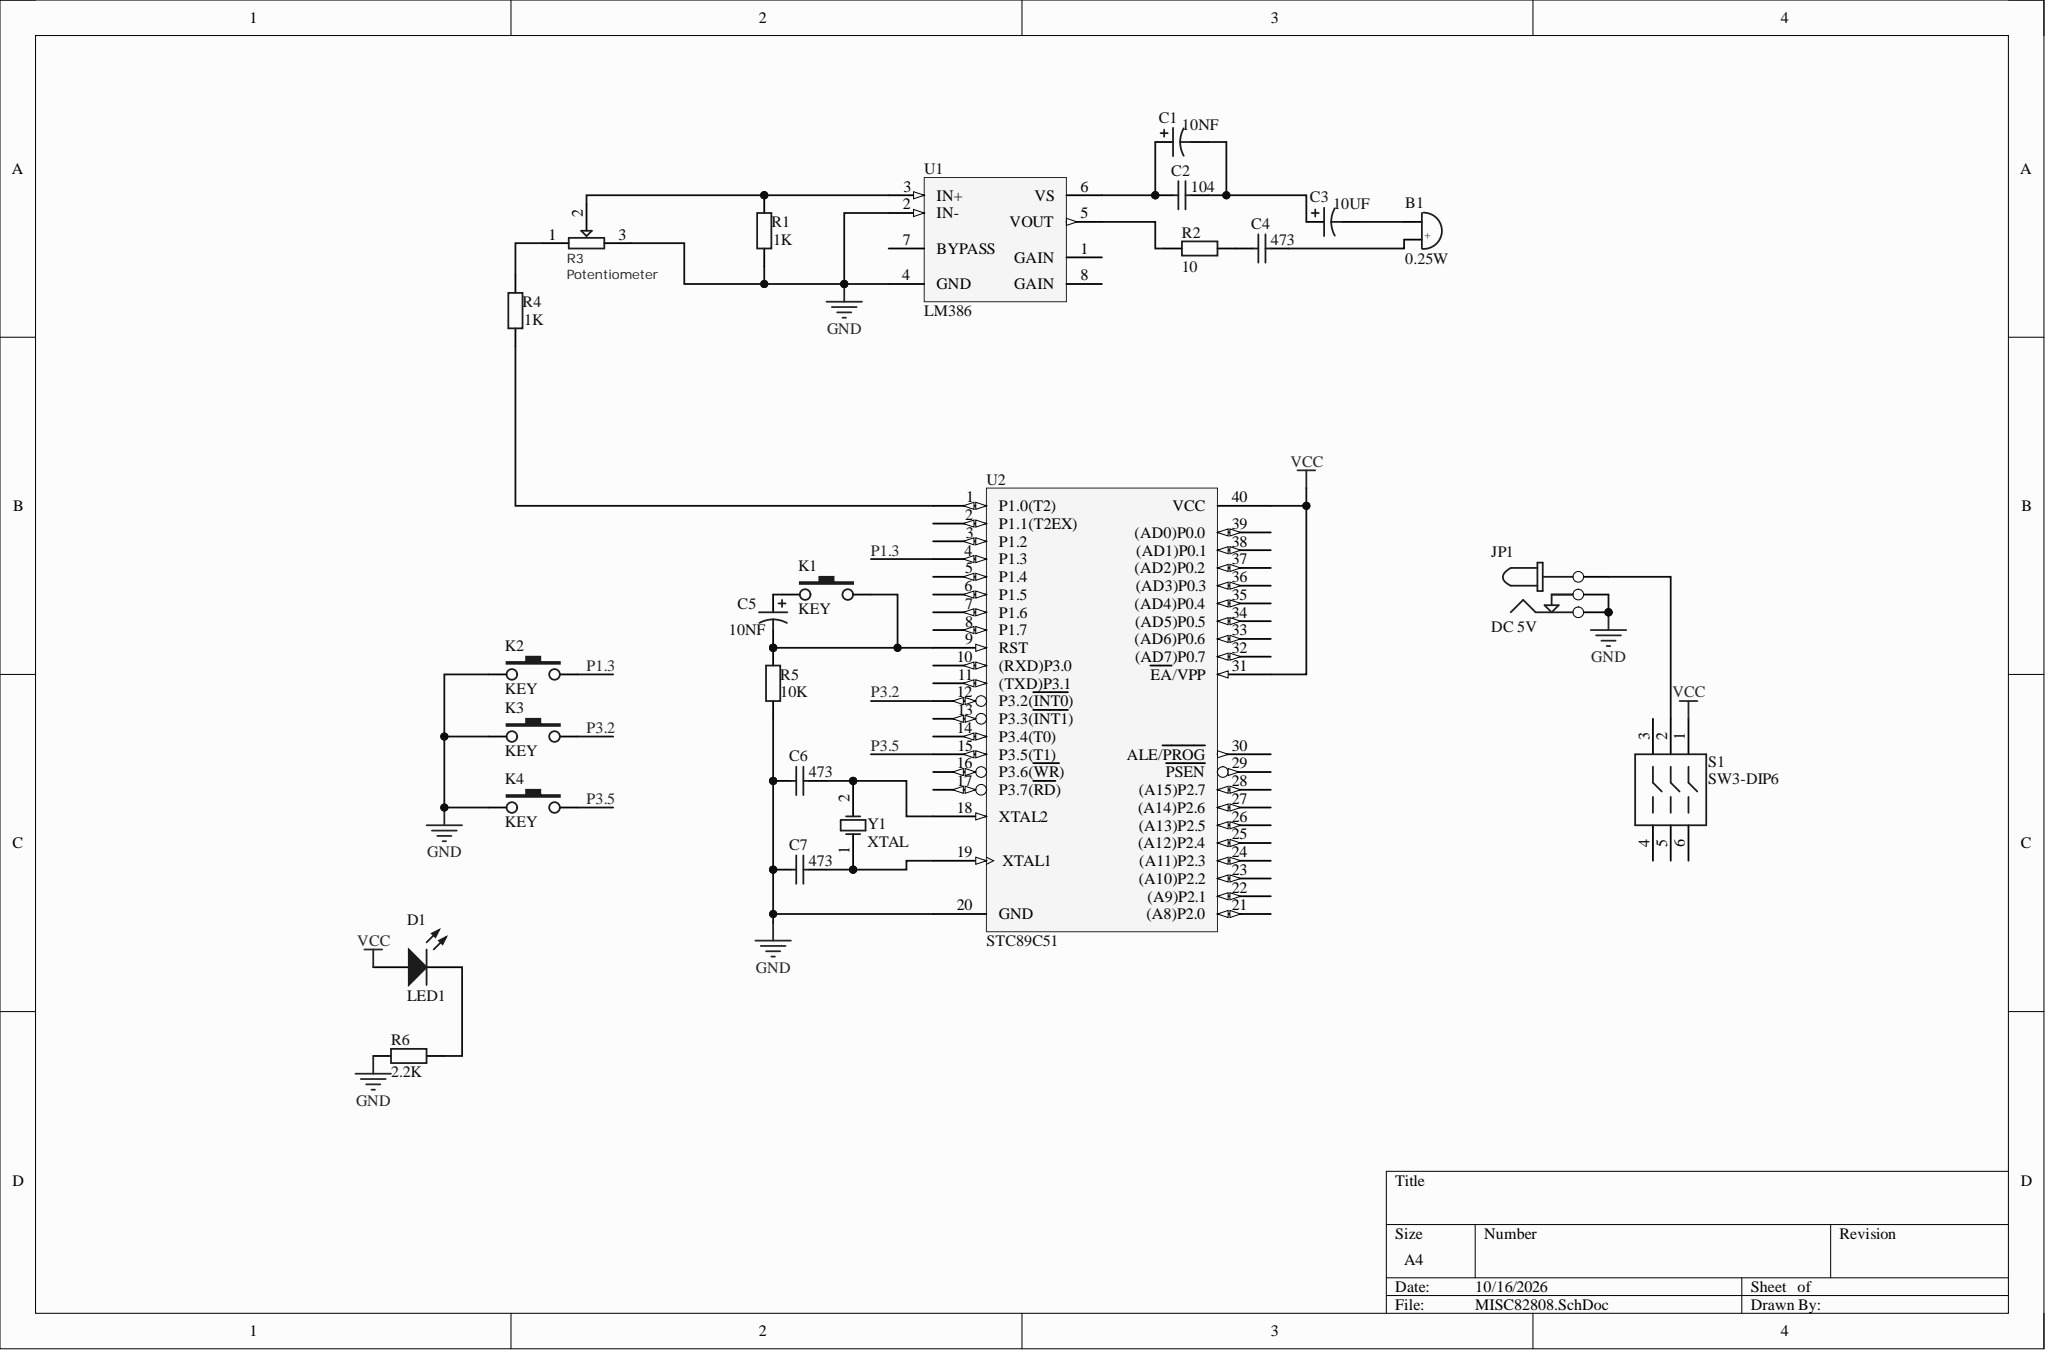Circuit board | Altium Designer | 24 parts | 20 nets
Bill of materials:
Comment,Description,Designator,Footprint,LibRef,Quantity
"0.25W","Buzzer","B1","BEEP 5x9x5.5","BEEP","1"
"Cap Pol1","Polarized Capacitor (Radial)","C1, C3, C5","RB7.6-15","Cap Pol1","3"
"Cap","Capacitor","C2, C4, C6, C7","RAD-0.3","Cap","4"
"LED1","Typical RED GaAs LED","D1","LED-1","LED1","1"
"DC 5V","DC power jack","JP1","DC POWER JACK1","DC POWER JACK1","1"
"KEY","","K1, K2, K3, K4","DIP-3X6X4.3","KEY","4"
"Res2","Resistor","R1, R2, R4, R5, R6","AXIAL-0.4","Res2","5"
"Potentiometer","","R3","滑动变阻器","滑动变阻器","1"
"SW3-DIP6","","S1","DIP-Switch3","SW3-DIP6","1"
"LM386","Low Voltage Audio Power Amplifier, 8-pin Narrow SOIC","U1","M08A_N","LM386M-1","1"
"STC89C51","","U2","DIP40","STC89C51","1"
"XTAL","Crystal Oscillator","Y1","R38","XTAL","1"
Netlist (Protel format):
[
B1
BEEP 5x9x5.5
0.25W



]
[
C1
RB7.6-15
Cap Pol1



]
[
C2
RAD-0.3
Cap



]
[
C3
RB7.6-15
Cap Pol1



]
[
C4
RAD-0.3
Cap



]
[
C5
RB7.6-15
Cap Pol1



]
[
C6
RAD-0.3
Cap



]
[
C7
RAD-0.3
Cap



]
[
D1
LED-1
LED1



]
[
JP1
DC POWER JACK1
DC 5V



]
[
K1
DIP-3X6X4.3
KEY



]
[
K2
DIP-3X6X4.3
KEY



]
[
K3
DIP-3X6X4.3
KEY



]
[
K4
DIP-3X6X4.3
KEY



]
[
R1
AXIAL-0.4
Res2



]
[
R2
AXIAL-0.4
Res2



]
[
R3
滑动变阻器
Potentiometer



]
[
R4
AXIAL-0.4
Res2



]
[
R5
AXIAL-0.4
Res2



]
[
R6
AXIAL-0.4
Res2



]
[
S1
DIP-Switch3
SW3-DIP6



]
[
U1
M08A_N
LM386



]
[
U2
DIP40
STC89C51



]
[
Y1
R38
XTAL



]
(
VCC
D1-1
S1-1
U2-31
U2-40
)
(
P3.5
K4-3
U2-15
)
(
P3.2
K3-3
U2-12
)
(
P1.3
K2-3
U2-4
)
(
NetR4_1
R4-1
U2-1
)
(
NetR3_1
R3-1
R4-2
)
(
NetR2_1
R2-1
U1-5
)
(
NetR1_2
R1-2
R3-2
U1-3
)
(
NetJP1_1
JP1-1
S1-2
)
(
NetD1_2
D1-2
R6-1
)
(
NetC7_2
C7-2
U2-19
Y1-1
)
(
NetC6_2
C6-2
U2-18
Y1-2
)
(
NetC5_2
C5-2
K1-3
R5-2
U2-9
)
(
NetC5_1
C5-1
K1-1
)
(
NetC4_1
C4-1
R2-2
)
(
NetC1_2
C1-2
C2-2
C3-1
)
(
NetC1_1
C1-1
C2-1
U1-6
)
(
NetB1_2
B1-2
C3-2
)
(
NetB1_1
B1-1
C4-2
)
(
GND
C6-1
C7-1
JP1-2
JP1-3
K2-1
K3-1
K4-1
R1-1
R3-3
R5-1
R6-2
U1-2
U1-4
U2-20
)